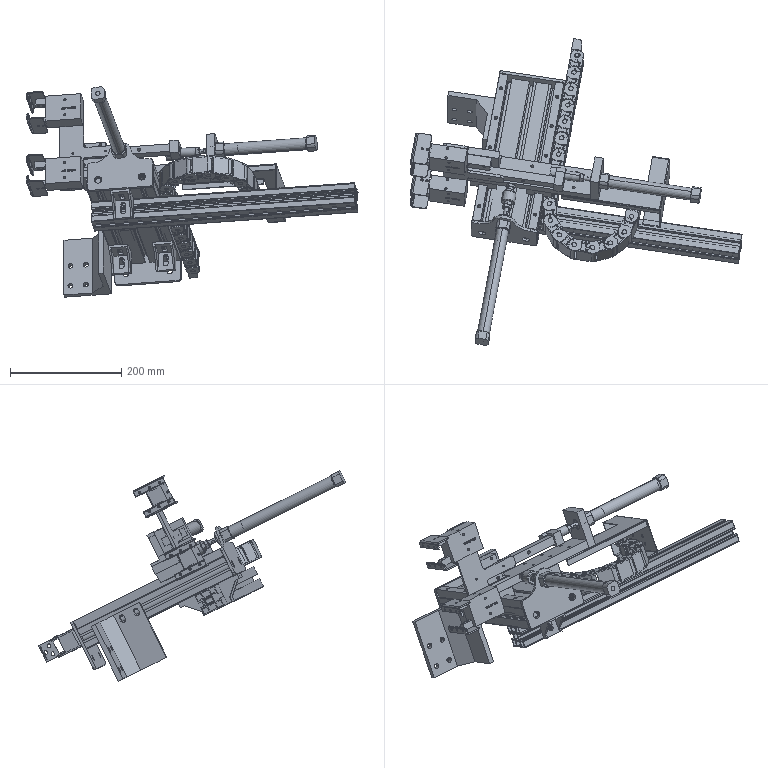Part | 64 solids | 4523 faces | volume 1993640 mm3 | plane 2567 | cylinder 1621 | spline 206 | cone 117 | torus 8 | sphere 4 | commonest cylinder face diameters 2 x204 1 x174 0.6 x138 23.26 x119 3.3 x104 11.94 x102